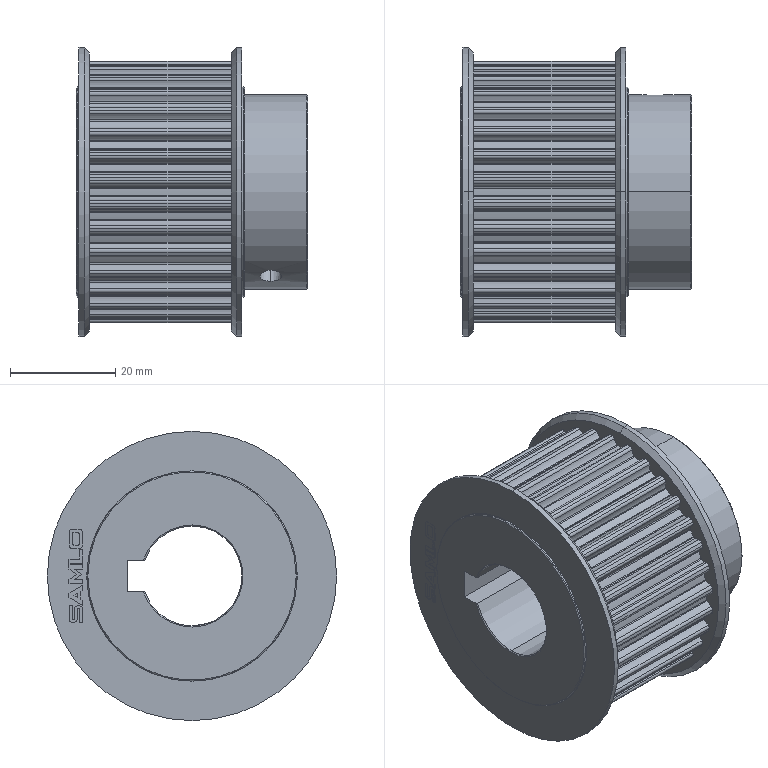Part | SolidWorks | features BaseBody 1 | 1 solid | 394 faces | box 44 x 55 x 55 mm | volume 58825 mm3 | cylinder 316 | plane 62 | cone 16 | commonest cylinder face diameters 1.1 x78 0.5 x74 6.55 x68 46.43 x33 49.97 x32 0.603 x4